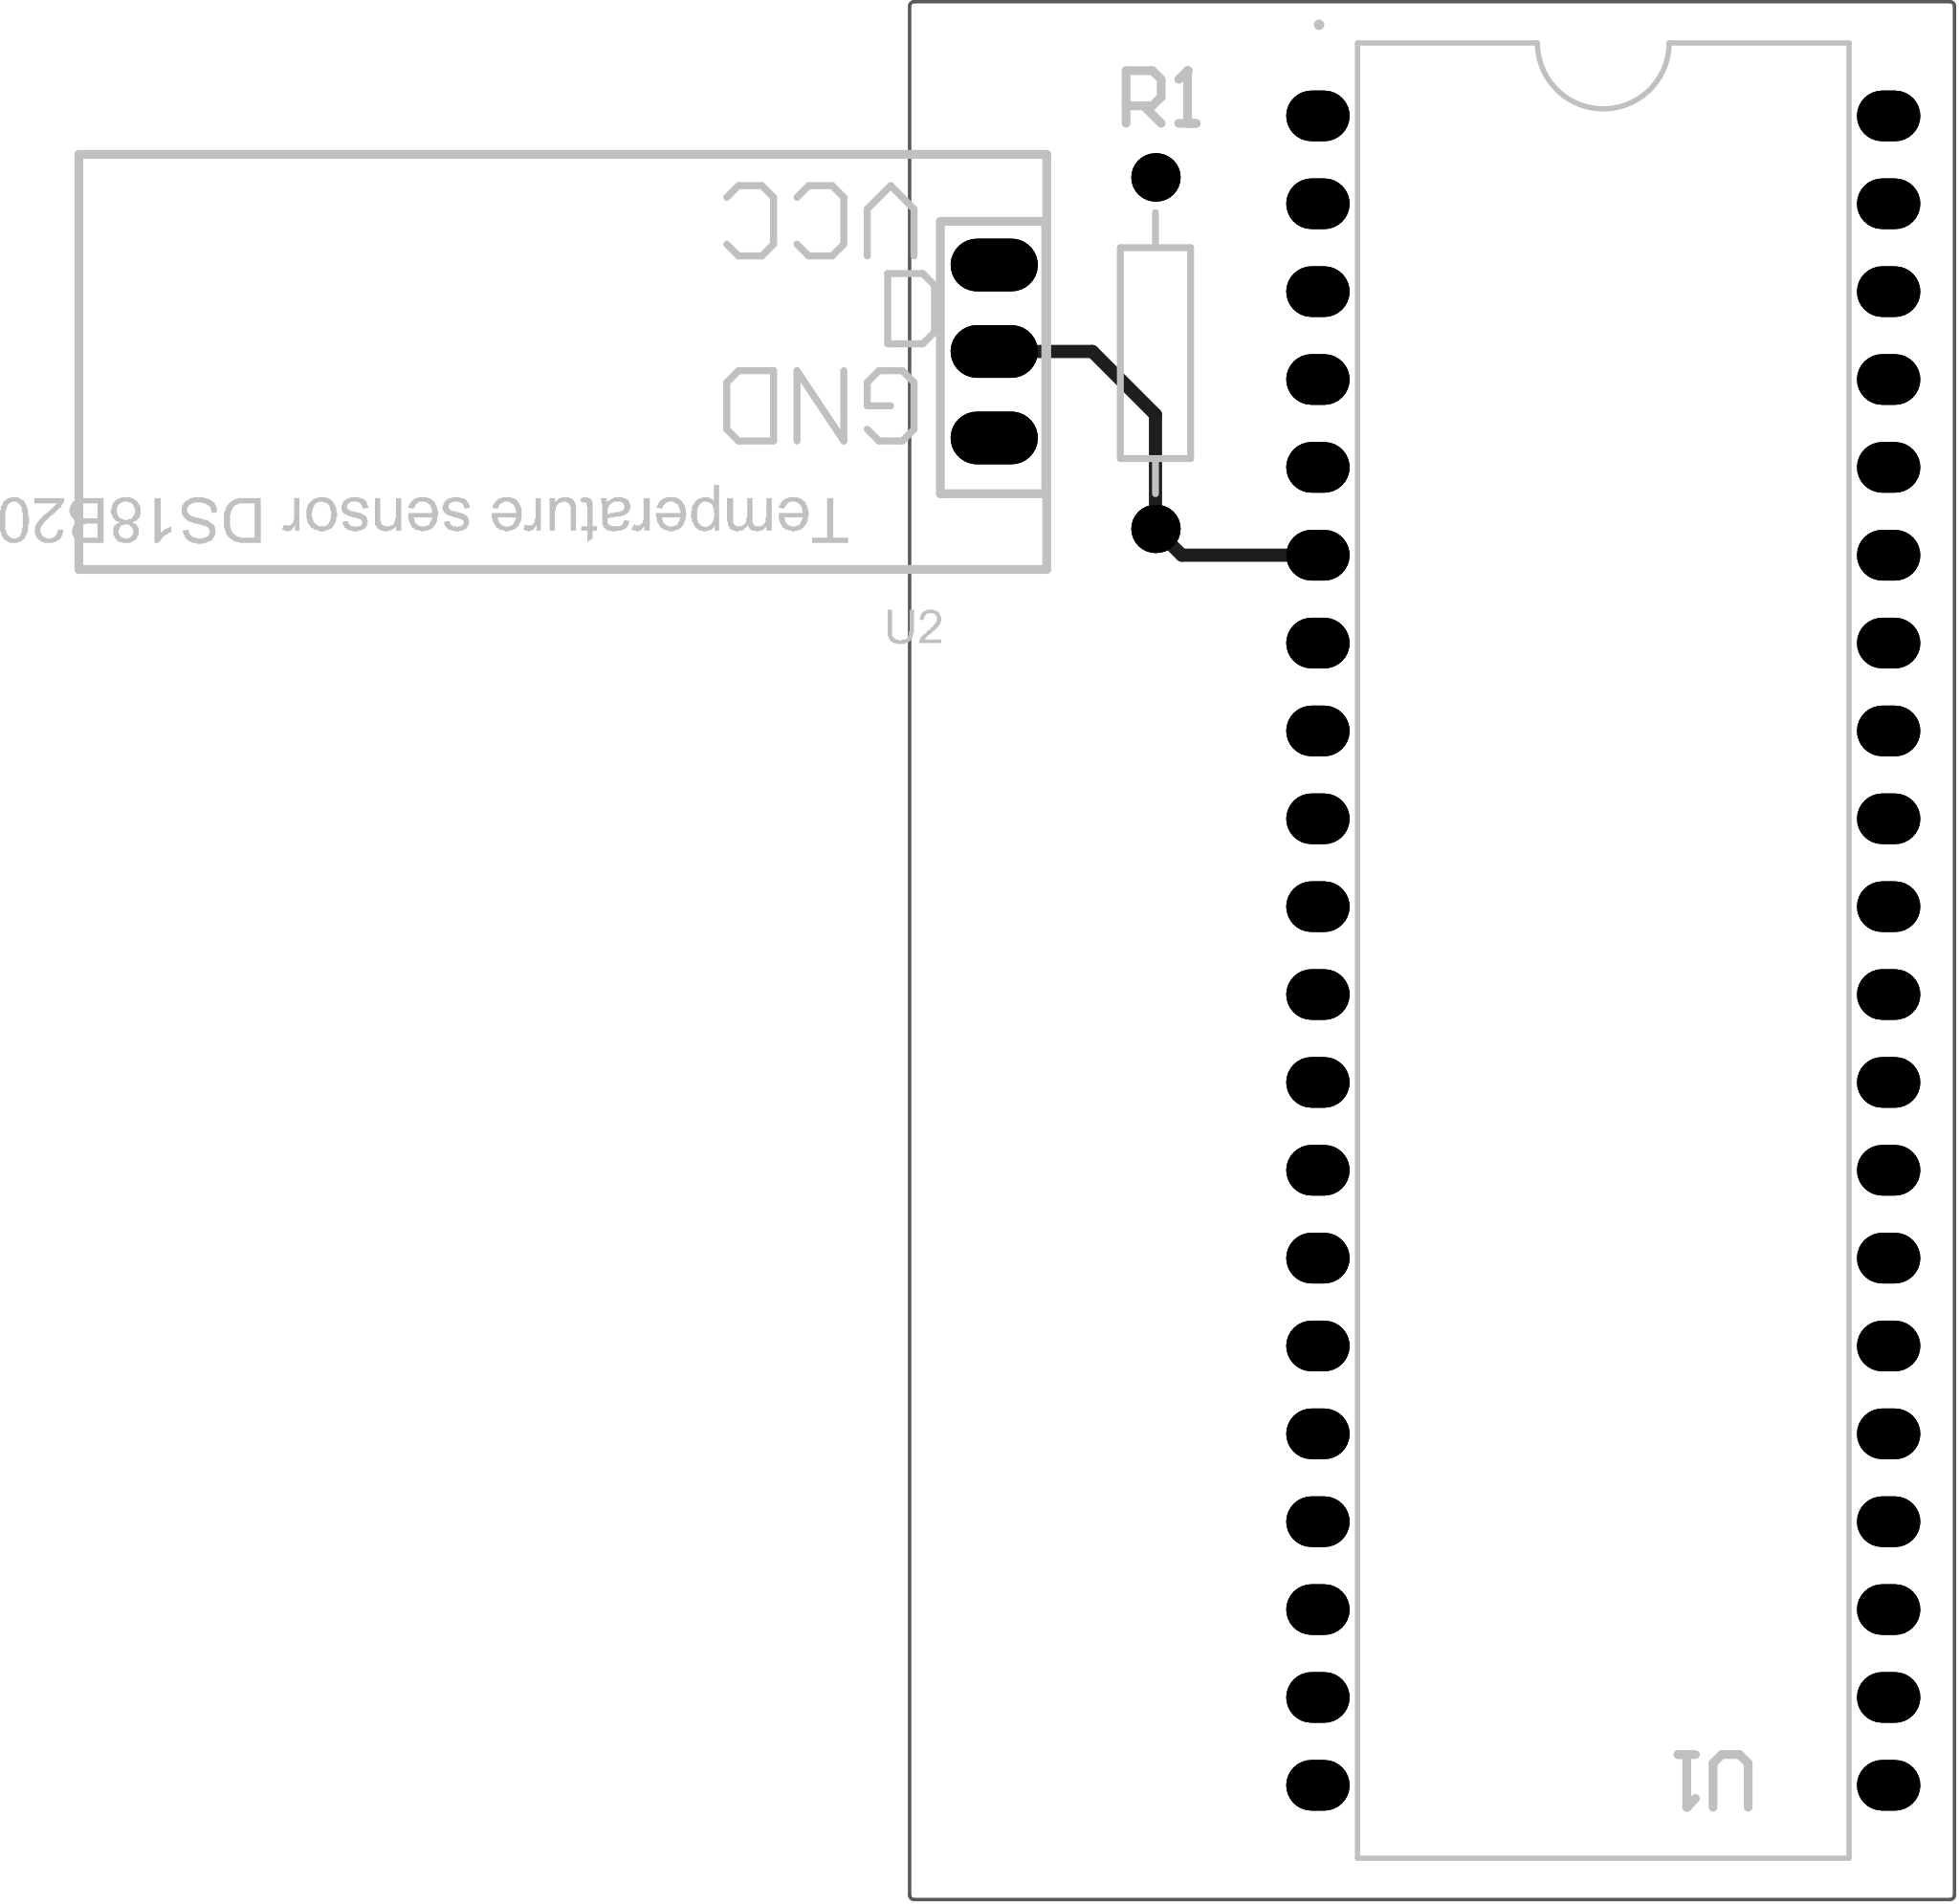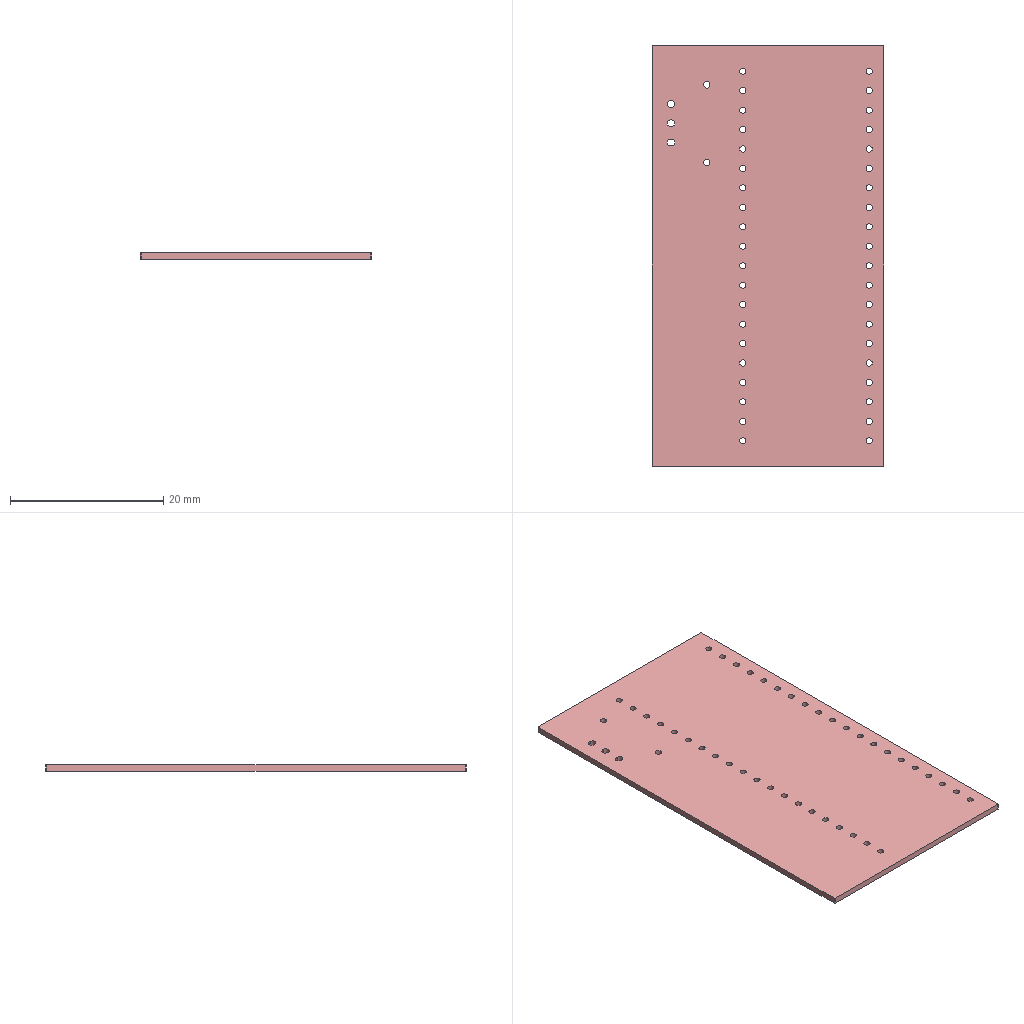Circuit board layout | Altium Designer | box 30.2 x 54.9 x 0.8 mm
Layer stack:
# Altium Designer layer stack of  (unit mm; dielectric type: 0 none, 1 core, 2 prepreg, 3 surface material)
index,name,kind,layer,copper_thickness_mm,dielectric_type,dielectric_thickness_mm,dielectric_material,dielectric_constant
0,Top Paste,other,,,,,,
1,Top Overlay,other,,,,,,
2,Top Solder,dielectric,,,3,0.0102,Solder Resist,3.5
3,Top Layer,copper,Top Layer,0.0356,,,,
4,Dielectric 1,dielectric,,,1,0.254,FR-4,4.2
5,GND,copper,GND,0.036,,,,
6,Dielectric 4,dielectric,,,2,0.127,,4.2
7,VCC,copper,VCC,0.036,,,,
8,Dielectric 3,dielectric,,,1,0.254,,4.2
9,Bottom Layer,copper,Bottom Layer,0.0356,,,,
10,Bottom Solder,dielectric,,,3,0.0102,Solder Resist,3.5
11,Bottom Overlay,other,,,,,,
12,Bottom Paste,other,,,,,,
# drill layer pairs: low layer,high layer
drill_pair,Top Layer,Bottom Layer
Part placement:
Designator,Comment,Layer,Footprint,Center-X(mm),Center-Y(mm),Rotation
U2,Comment,TopLayer,DS18B20,77.885,90.98,180
U1,STC89C52RC,TopLayer,STC89C52RC,95.504,73.66,270
R1,10K,TopLayer,AXIAL-0.4,82.55,90.932,90
Pad and via stacks:
# Altium Designer via and pad stacks of  (unit mm). Each distinct definition once, with the count of objects using it.
# via: kind,start_layer,end_layer,hole_mm,diameter_mm,mode(0 simple;1 top-mid-bottom;2 full stack),diameter_per_layer,count,example_net
# pad: kind,layer,hole_mm,hole_type(0 round;1 square;2 slot),plating,top_size,top_shape(1 round;2 rect;3 octagon;9 rounded rect),mid_size,bottom_size,mode,footprint,size_per_layer,count,example
pad,Multi-Layer,0.9,2,plated,2.524x1.524,1,2.524x1.524,2.524x1.524,0,DS18B20,,3,U2.2
pad,Multi-Layer,0.8,0,plated,1.467x1.833,1,1.467x1.833,1.467x1.833,0,STC89C52RC,,40,U1.21
pad,Multi-Layer,0.85,0,plated,1.4x1.4,1,1.4x1.4,1.4x1.4,0,AXIAL-0.4,,2,R1.1
Design rules, without the lines most boards share:
# Altium Designer design rules of  (exported by Altium Designer, unit mm)
# columns: name | kind | enabled | priority | scope1 | scope2 | descriptor | typed fields (field=value)
SilkToSilkClearance | 55 | enabled | 1 | All | All | Silk to Silk (Clearance=0mil) (All),(All) |
SilkToSolderMaskClearance | 54 | enabled | 1 | IsPad | All | Silk To Solder Mask (Clearance=0mil) (IsPad),(All) |
MinimumSolderMaskSliver | 53 | enabled | 1 | All | All | Minimum Solder Mask Sliver (Gap=0mil) (All),(All) |
HoleToHoleClearance | 52 | enabled | 1 | All | All | Hole To Hole Clearance (Gap=10mil) (All),(All) | gap=0.254
DiffPairsRouting | 51 | enabled | 1 | All | All | Differential Pairs Uncoupled Length using the Gap Constraints (Min=10mil) (Max=10mil) (Prefered=10mil)  and Width Constraints (Min=15mil) (Max=15mil) (Prefered=15mil) (All) |
SolderMaskExpansion | 13 | enabled | 1 | All | All | Solder Mask Expansion (Expansion =4mil) (All) | expansion=0.1016
PasteMaskExpansion | 14 | enabled | 1 | All | All | Paste Mask Expansion (Expansion =0mil) (All) | expansion=0
RoutingVias | 11 | enabled | 1 | All | All | Routing Via (MinHoleWidth=28mil) (MaxHoleWidth=28mil) (PreferredHoleWidth=28mil) (MinWidth=50mil) (MaxWidth=50mil) (PreferedWidth=50mil) (All) | via_min_hole=0.7112 via_max_hole=0.7112 via_preferred_diameter=1.27 via_preferred_hole=0.7112
Width | 2 | enabled | 1 | All | All | Width Constraint (Min=10mil) (Max=30mil) (Preferred=10mil) (All) |
PolygonConnect | 20 | enabled | 1 | All | All | Polygon Connect Rule(Relief Connect )(Conductor Width=10mil) (Relief Angle=90 Angle) (Entries=4) (Air Gap Width=10mil) (All),(All) | connect_style(0=relief,1=direct,2=none)=0 relief_conductor_width=0.254 relief_entries=4
PlaneConnect | 6 | enabled | 1 | All | All | Power Plane Connect Rule(Relief Connect )(Expansion=20mil) (Conductor Width=10mil) (Air Gap=10mil) (Entries=4) (All) | relief_conductor_width=0.254 relief_entries=4 relief_expansion=0.508
Clearance | 0 | enabled | 1 | All | All | Clearance Constraint (Gap=10mil) (All),(All) | gap=0.254
Classes set for this board:
# Altium Designer classes of  (member kind: 0 net, 1 component, 2 from-to, 3 pad, 4 layer, 5 differential pair, 6 design channel, 7 polygon, 8 structure, 9 xSignal)
# columns: class name | member kind | superclass | members
Sheet1 | 1 | no | R1; U1; U2;